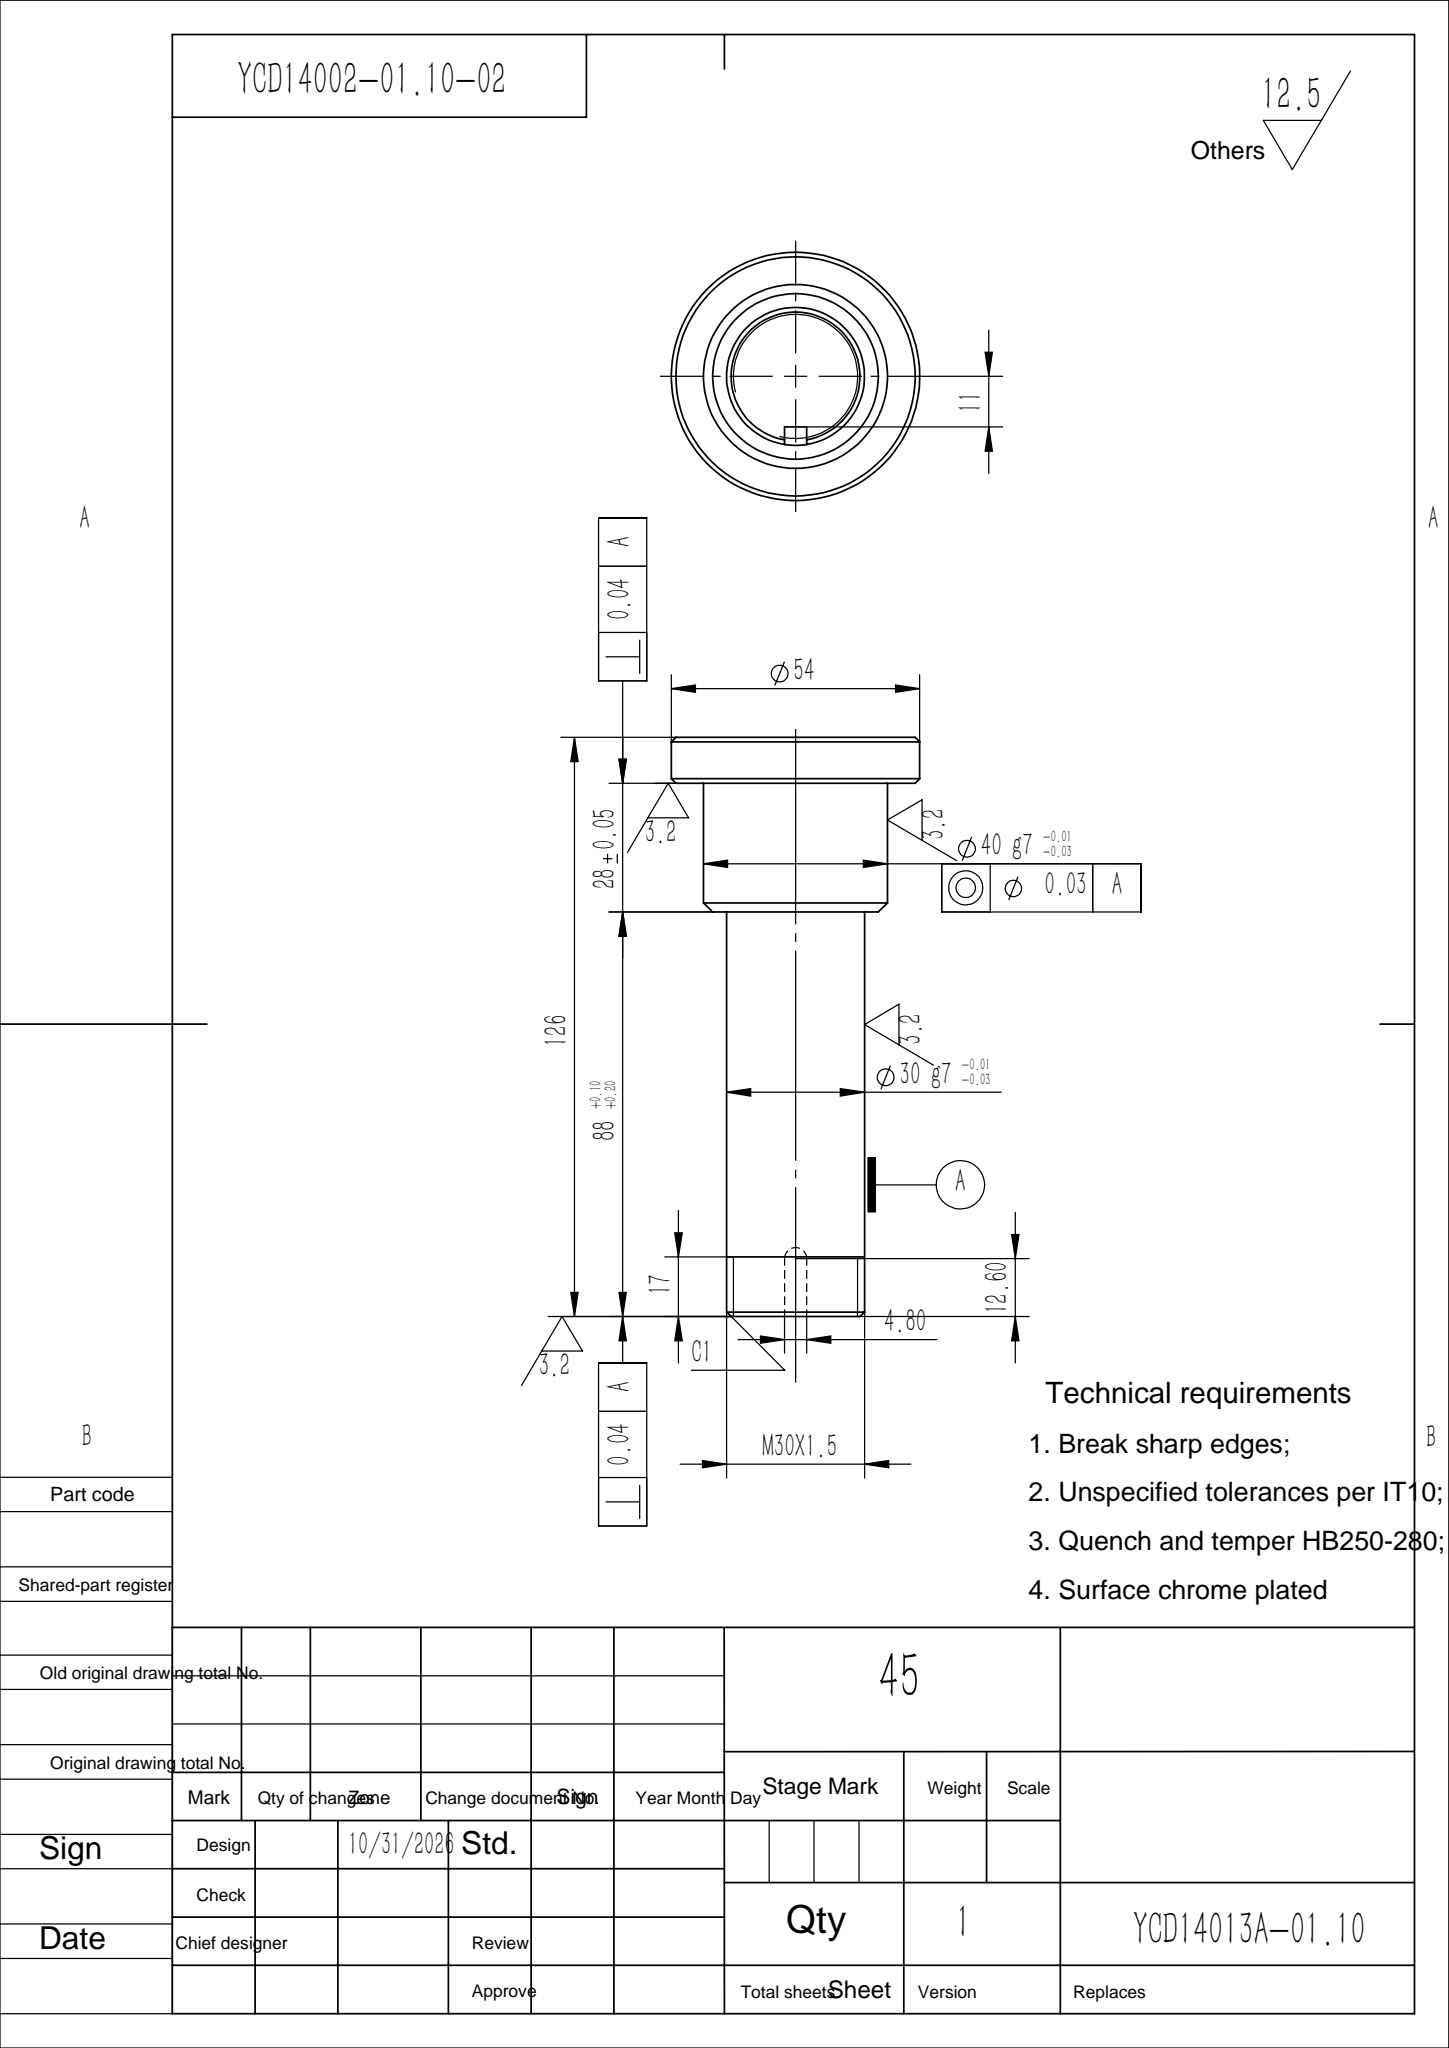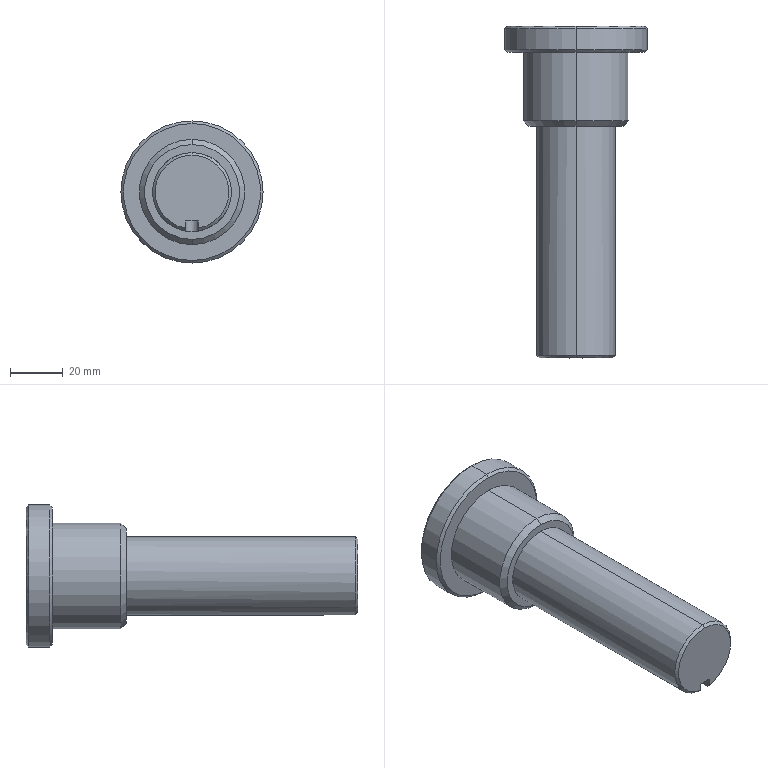Part | SolidWorks | features ICE 4, Chamfer 2, Extrusion 1 | 1 solid | 22 faces | box 54 x 126 x 54 mm | volume 119564 mm3 | cone 8 | cylinder 7 | plane 7 | commonest cylinder face diameters 30 x2 40 x2 54 x2 4.8 x1
STEP:
#1=CARTESIAN_POINT('',(0.,0.,-18.));
#2=VERTEX_POINT('',#1);
#3=CARTESIAN_POINT('',(0.,0.,18.));
#4=VERTEX_POINT('',#3);
#5=CARTESIAN_POINT('',(0.,0.,0.));
#6=DIRECTION('',(0.,-1.,0.));
#7=DIRECTION('',(0.,0.,1.));
#8=AXIS2_PLACEMENT_3D('',#5,#6,#7);
#9=CIRCLE('',#8,18.);
#10=EDGE_CURVE('',#2,#4,#9,.T.);
#11=ORIENTED_EDGE('',*,*,#10,.F.);
#12=CARTESIAN_POINT('',(0.,2.,-20.));
#13=VERTEX_POINT('',#12);
#14=CARTESIAN_POINT('',(0.,2.,-20.));
#15=DIRECTION('',(0.,0.7071,-0.7071));
#16=VECTOR('',#15,1000.);
#17=LINE('',#14,#16);
#18=EDGE_CURVE('',#2,#13,#17,.T.);
#19=ORIENTED_EDGE('',*,*,#18,.T.);
#20=CARTESIAN_POINT('',(0.,2.,20.));
#21=VERTEX_POINT('',#20);
#22=CARTESIAN_POINT('',(0.,2.,0.));
#23=DIRECTION('',(0.,1.,0.));
#24=DIRECTION('',(0.,0.,1.));
#25=AXIS2_PLACEMENT_3D('',#22,#23,#24);
#26=CIRCLE('',#25,20.);
#27=EDGE_CURVE('',#21,#13,#26,.T.);
#28=ORIENTED_EDGE('',*,*,#27,.F.);
#29=CARTESIAN_POINT('',(0.,2.,20.));
#30=DIRECTION('',(0.,0.7071,0.7071));
#31=VECTOR('',#30,1000.);
#32=LINE('',#29,#31);
#33=EDGE_CURVE('',#4,#21,#32,.T.);
#34=ORIENTED_EDGE('',*,*,#33,.F.);
#35=EDGE_LOOP('',(#11,#19,#28,#34));
#36=FACE_OUTER_BOUND('',#35,.T.);
#37=CARTESIAN_POINT('',(0.,2.,0.));
#38=DIRECTION('',(0.,1.,0.));
#39=DIRECTION('',(0.,0.,1.));
#40=AXIS2_PLACEMENT_3D('',#37,#38,#39);
#41=CONICAL_SURFACE('',#40,20.,0.7854);
#42=ADVANCED_FACE('',(#36),#41,.T.);
#43=CARTESIAN_POINT('',(0.,38.,26.));
#44=VERTEX_POINT('',#43);
#45=CARTESIAN_POINT('',(0.,38.,-26.));
#46=VERTEX_POINT('',#45);
#47=CARTESIAN_POINT('',(0.,38.,0.));
#48=DIRECTION('',(0.,1.,0.));
#49=DIRECTION('',(0.,0.,1.));
#50=AXIS2_PLACEMENT_3D('',#47,#48,#49);
#51=CIRCLE('',#50,26.);
#52=EDGE_CURVE('',#44,#46,#51,.T.);
#53=ORIENTED_EDGE('',*,*,#52,.F.);
#54=CARTESIAN_POINT('',(0.,37.,27.));
#55=VERTEX_POINT('',#54);
#56=CARTESIAN_POINT('',(0.,38.,26.));
#57=DIRECTION('',(0.,-0.7071,0.7071));
#58=VECTOR('',#57,1000.);
#59=LINE('',#56,#58);
#60=EDGE_CURVE('',#44,#55,#59,.T.);
#61=ORIENTED_EDGE('',*,*,#60,.T.);
#62=CARTESIAN_POINT('',(0.,37.,-27.));
#63=VERTEX_POINT('',#62);
#64=CARTESIAN_POINT('',(0.,37.,0.));
#65=DIRECTION('',(0.,-1.,0.));
#66=DIRECTION('',(0.,0.,1.));
#67=AXIS2_PLACEMENT_3D('',#64,#65,#66);
#68=CIRCLE('',#67,27.);
#69=EDGE_CURVE('',#63,#55,#68,.T.);
#70=ORIENTED_EDGE('',*,*,#69,.F.);
#71=CARTESIAN_POINT('',(0.,38.,-26.));
#72=DIRECTION('',(0.,-0.7071,-0.7071));
#73=VECTOR('',#72,1000.);
#74=LINE('',#71,#73);
#75=EDGE_CURVE('',#46,#63,#74,.T.);
#76=ORIENTED_EDGE('',*,*,#75,.F.);
#77=EDGE_LOOP('',(#53,#61,#70,#76));
#78=FACE_OUTER_BOUND('',#77,.T.);
#79=CARTESIAN_POINT('',(0.,38.,0.));
#80=DIRECTION('',(0.,-1.,0.));
#81=DIRECTION('',(0.,0.,-1.));
#82=AXIS2_PLACEMENT_3D('',#79,#80,#81);
#83=CONICAL_SURFACE('',#82,26.,0.7854);
#84=ADVANCED_FACE('',(#78),#83,.T.);
#85=CARTESIAN_POINT('',(0.,28.,-26.));
#86=VERTEX_POINT('',#85);
#87=CARTESIAN_POINT('',(0.,28.,26.));
#88=VERTEX_POINT('',#87);
#89=CARTESIAN_POINT('',(0.,28.,0.));
#90=DIRECTION('',(0.,-1.,0.));
#91=DIRECTION('',(0.,0.,1.));
#92=AXIS2_PLACEMENT_3D('',#89,#90,#91);
#93=CIRCLE('',#92,26.);
#94=EDGE_CURVE('',#86,#88,#93,.T.);
#95=ORIENTED_EDGE('',*,*,#94,.F.);
#96=CARTESIAN_POINT('',(0.,29.,-27.));
#97=VERTEX_POINT('',#96);
#98=CARTESIAN_POINT('',(0.,29.,-27.));
#99=DIRECTION('',(0.,0.7071,-0.7071));
#100=VECTOR('',#99,1000.);
#101=LINE('',#98,#100);
#102=EDGE_CURVE('',#86,#97,#101,.T.);
#103=ORIENTED_EDGE('',*,*,#102,.T.);
#104=CARTESIAN_POINT('',(0.,29.,27.));
#105=VERTEX_POINT('',#104);
#106=CARTESIAN_POINT('',(0.,29.,0.));
#107=DIRECTION('',(0.,1.,0.));
#108=DIRECTION('',(0.,0.,1.));
#109=AXIS2_PLACEMENT_3D('',#106,#107,#108);
#110=CIRCLE('',#109,27.);
#111=EDGE_CURVE('',#105,#97,#110,.T.);
#112=ORIENTED_EDGE('',*,*,#111,.F.);
#113=CARTESIAN_POINT('',(0.,29.,27.));
#114=DIRECTION('',(0.,0.7071,0.7071));
#115=VECTOR('',#114,1000.);
#116=LINE('',#113,#115);
#117=EDGE_CURVE('',#88,#105,#116,.T.);
#118=ORIENTED_EDGE('',*,*,#117,.F.);
#119=EDGE_LOOP('',(#95,#103,#112,#118));
#120=FACE_OUTER_BOUND('',#119,.T.);
#121=CARTESIAN_POINT('',(0.,29.,0.));
#122=DIRECTION('',(0.,1.,0.));
#123=DIRECTION('',(0.,0.,1.));
#124=AXIS2_PLACEMENT_3D('',#121,#122,#123);
#125=CONICAL_SURFACE('',#124,27.,0.7854);
#126=ADVANCED_FACE('',(#120),#125,.T.);
#127=CARTESIAN_POINT('',(0.,-88.,14.));
#128=VERTEX_POINT('',#127);
#129=CARTESIAN_POINT('',(-2.4,-88.,-13.793));
#130=VERTEX_POINT('',#129);
#131=CARTESIAN_POINT('',(0.,-88.,0.));
#132=DIRECTION('',(0.,-1.,0.));
#133=DIRECTION('',(0.,0.,-1.));
#134=AXIS2_PLACEMENT_3D('',#131,#132,#133);
#135=CIRCLE('',#134,14.);
#136=EDGE_CURVE('',#128,#130,#135,.T.);
#137=ORIENTED_EDGE('',*,*,#136,.F.);
#138=CARTESIAN_POINT('',(0.,-87.,15.));
#139=VERTEX_POINT('',#138);
#140=CARTESIAN_POINT('',(0.,-88.,14.));
#141=DIRECTION('',(0.,0.7071,0.7071));
#142=VECTOR('',#141,1000.);
#143=LINE('',#140,#142);
#144=EDGE_CURVE('',#128,#139,#143,.T.);
#145=ORIENTED_EDGE('',*,*,#144,.T.);
#146=CARTESIAN_POINT('',(-2.4,-87.,-14.807));
#147=VERTEX_POINT('',#146);
#148=CARTESIAN_POINT('',(0.,-87.,0.));
#149=DIRECTION('',(0.,1.,0.));
#150=DIRECTION('',(0.,0.,-1.));
#151=AXIS2_PLACEMENT_3D('',#148,#149,#150);
#152=CIRCLE('',#151,15.);
#153=EDGE_CURVE('',#147,#139,#152,.T.);
#154=ORIENTED_EDGE('',*,*,#153,.F.);
#155=CARTESIAN_POINT('',(-2.4,-88.,-13.793));
#156=CARTESIAN_POINT('',(-2.4,-87.667,-14.131));
#157=CARTESIAN_POINT('',(-2.4,-87.333,-14.469));
#158=CARTESIAN_POINT('',(-2.4,-87.,-14.807));
#159=B_SPLINE_CURVE_WITH_KNOTS('',3,(#155,#156,#157,#158),.UNSPECIFIED.,.F.,.F.,(4,4),(0.006945,0.00837),.UNSPECIFIED.);
#160=EDGE_CURVE('',#130,#147,#159,.T.);
#161=ORIENTED_EDGE('',*,*,#160,.F.);
#162=EDGE_LOOP('',(#137,#145,#154,#161));
#163=FACE_OUTER_BOUND('',#162,.T.);
#164=CARTESIAN_POINT('',(0.,-88.,0.));
#165=DIRECTION('',(0.,1.,0.));
#166=DIRECTION('',(0.,0.,1.));
#167=AXIS2_PLACEMENT_3D('',#164,#165,#166);
#168=CONICAL_SURFACE('',#167,14.,0.7854);
#169=ADVANCED_FACE('',(#163),#168,.T.);
#170=CARTESIAN_POINT('',(2.4,-75.4,-14.807));
#171=VERTEX_POINT('',#170);
#172=CARTESIAN_POINT('',(0.,-73.,-15.));
#173=VERTEX_POINT('',#172);
#174=CARTESIAN_POINT('',(2.4,-75.4,-14.807));
#175=CARTESIAN_POINT('',(2.4,-75.241,-14.807));
#176=CARTESIAN_POINT('',(2.384,-75.085,-14.809));
#177=CARTESIAN_POINT('',(2.323,-74.778,-14.819));
#178=CARTESIAN_POINT('',(2.277,-74.625,-14.826));
#179=CARTESIAN_POINT('',(2.156,-74.335,-14.844));
#180=CARTESIAN_POINT('',(2.083,-74.197,-14.855));
#181=CARTESIAN_POINT('',(1.908,-73.936,-14.878));
#182=CARTESIAN_POINT('',(1.807,-73.813,-14.891));
#183=CARTESIAN_POINT('',(1.475,-73.481,-14.929));
#184=CARTESIAN_POINT('',(1.208,-73.303,-14.954));
#185=CARTESIAN_POINT('',(0.7745,-73.123,-14.981));
#186=CARTESIAN_POINT('',(0.6228,-73.077,-14.988));
#187=CARTESIAN_POINT('',(0.3128,-73.015,-14.998));
#188=CARTESIAN_POINT('',(0.1569,-73.,-15.));
#189=CARTESIAN_POINT('',(0.,-73.,-15.));
#190=B_SPLINE_CURVE_WITH_KNOTS('',3,(#174,#175,#176,#177,#178,#179,#180,#181,#182,#183,#184,#185,#186,#187,#188,#189),.UNSPECIFIED.,.F.,.F.,(4,2,2,2,2,2,2,4),(0.,0.0004698,0.0009397,0.00141,0.001879,0.002819,0.003289,0.003759),.UNSPECIFIED.);
#191=EDGE_CURVE('',#171,#173,#190,.T.);
#192=ORIENTED_EDGE('',*,*,#191,.T.);
#193=CARTESIAN_POINT('',(0.,0.,-15.));
#194=VERTEX_POINT('',#193);
#195=CARTESIAN_POINT('',(0.,-88.,-15.));
#196=DIRECTION('',(0.,1.,0.));
#197=VECTOR('',#196,1000.);
#198=LINE('',#195,#197);
#199=EDGE_CURVE('',#173,#194,#198,.T.);
#200=ORIENTED_EDGE('',*,*,#199,.T.);
#201=CARTESIAN_POINT('',(0.,0.,15.));
#202=VERTEX_POINT('',#201);
#203=CARTESIAN_POINT('',(0.,0.,0.));
#204=DIRECTION('',(0.,-1.,0.));
#205=DIRECTION('',(0.,0.,1.));
#206=AXIS2_PLACEMENT_3D('',#203,#204,#205);
#207=CIRCLE('',#206,15.);
#208=EDGE_CURVE('',#194,#202,#207,.T.);
#209=ORIENTED_EDGE('',*,*,#208,.T.);
#210=CARTESIAN_POINT('',(0.,-88.,15.));
#211=DIRECTION('',(0.,1.,0.));
#212=VECTOR('',#211,1000.);
#213=LINE('',#210,#212);
#214=EDGE_CURVE('',#139,#202,#213,.T.);
#215=ORIENTED_EDGE('',*,*,#214,.F.);
#216=CARTESIAN_POINT('',(2.4,-87.,-14.807));
#217=VERTEX_POINT('',#216);
#218=CARTESIAN_POINT('',(0.,-87.,0.));
#219=DIRECTION('',(0.,1.,0.));
#220=DIRECTION('',(0.,0.,-1.));
#221=AXIS2_PLACEMENT_3D('',#218,#219,#220);
#222=CIRCLE('',#221,15.);
#223=EDGE_CURVE('',#139,#217,#222,.T.);
#224=ORIENTED_EDGE('',*,*,#223,.T.);
#225=CARTESIAN_POINT('',(2.4,-88.,-14.807));
#226=DIRECTION('',(0.,1.,0.));
#227=VECTOR('',#226,1000.);
#228=LINE('',#225,#227);
#229=EDGE_CURVE('',#217,#171,#228,.T.);
#230=ORIENTED_EDGE('',*,*,#229,.T.);
#231=EDGE_LOOP('',(#192,#200,#209,#215,#224,#230));
#232=FACE_OUTER_BOUND('',#231,.T.);
#233=CARTESIAN_POINT('',(0.,-88.,0.));
#234=DIRECTION('',(0.,1.,0.));
#235=DIRECTION('',(0.,0.,1.));
#236=AXIS2_PLACEMENT_3D('',#233,#234,#235);
#237=CYLINDRICAL_SURFACE('',#236,15.);
#238=ADVANCED_FACE('',(#232),#237,.T.);
#239=ORIENTED_EDGE('',*,*,#69,.T.);
#240=CARTESIAN_POINT('',(0.,38.,27.));
#241=DIRECTION('',(0.,-1.,0.));
#242=VECTOR('',#241,1000.);
#243=LINE('',#240,#242);
#244=EDGE_CURVE('',#55,#105,#243,.T.);
#245=ORIENTED_EDGE('',*,*,#244,.T.);
#246=ORIENTED_EDGE('',*,*,#111,.T.);
#247=CARTESIAN_POINT('',(0.,38.,-27.));
#248=DIRECTION('',(0.,-1.,0.));
#249=VECTOR('',#248,1000.);
#250=LINE('',#247,#249);
#251=EDGE_CURVE('',#63,#97,#250,.T.);
#252=ORIENTED_EDGE('',*,*,#251,.F.);
#253=EDGE_LOOP('',(#239,#245,#246,#252));
#254=FACE_OUTER_BOUND('',#253,.T.);
#255=CARTESIAN_POINT('',(0.,38.,0.));
#256=DIRECTION('',(0.,-1.,0.));
#257=DIRECTION('',(0.,0.,-1.));
#258=AXIS2_PLACEMENT_3D('',#255,#256,#257);
#259=CYLINDRICAL_SURFACE('',#258,27.);
#260=ADVANCED_FACE('',(#254),#259,.T.);
#261=CARTESIAN_POINT('',(0.,28.,20.));
#262=VERTEX_POINT('',#261);
#263=CARTESIAN_POINT('',(0.,28.,-20.));
#264=VERTEX_POINT('',#263);
#265=CARTESIAN_POINT('',(0.,28.,0.));
#266=DIRECTION('',(0.,1.,0.));
#267=DIRECTION('',(0.,0.,1.));
#268=AXIS2_PLACEMENT_3D('',#265,#266,#267);
#269=CIRCLE('',#268,20.);
#270=EDGE_CURVE('',#262,#264,#269,.T.);
#271=ORIENTED_EDGE('',*,*,#270,.F.);
#272=CARTESIAN_POINT('',(0.,28.,20.));
#273=DIRECTION('',(0.,-1.,0.));
#274=VECTOR('',#273,1000.);
#275=LINE('',#272,#274);
#276=EDGE_CURVE('',#262,#21,#275,.T.);
#277=ORIENTED_EDGE('',*,*,#276,.T.);
#278=ORIENTED_EDGE('',*,*,#27,.T.);
#279=CARTESIAN_POINT('',(0.,28.,-20.));
#280=DIRECTION('',(0.,-1.,0.));
#281=VECTOR('',#280,1000.);
#282=LINE('',#279,#281);
#283=EDGE_CURVE('',#264,#13,#282,.T.);
#284=ORIENTED_EDGE('',*,*,#283,.F.);
#285=EDGE_LOOP('',(#271,#277,#278,#284));
#286=FACE_OUTER_BOUND('',#285,.T.);
#287=CARTESIAN_POINT('',(0.,28.,0.));
#288=DIRECTION('',(0.,-1.,0.));
#289=DIRECTION('',(0.,0.,-1.));
#290=AXIS2_PLACEMENT_3D('',#287,#288,#289);
#291=CYLINDRICAL_SURFACE('',#290,20.);
#292=ADVANCED_FACE('',(#286),#291,.T.);
#293=CARTESIAN_POINT('',(0.,0.,0.));
#294=DIRECTION('',(0.,-1.,0.));
#295=DIRECTION('',(0.,0.,1.));
#296=AXIS2_PLACEMENT_3D('',#293,#294,#295);
#297=CIRCLE('',#296,18.);
#298=EDGE_CURVE('',#4,#2,#297,.T.);
#299=ORIENTED_EDGE('',*,*,#298,.T.);
#300=ORIENTED_EDGE('',*,*,#10,.T.);
#301=EDGE_LOOP('',(#299,#300));
#302=FACE_OUTER_BOUND('',#301,.T.);
#303=CARTESIAN_POINT('',(0.,0.,0.));
#304=DIRECTION('',(0.,-1.,0.));
#305=DIRECTION('',(0.,0.,1.));
#306=AXIS2_PLACEMENT_3D('',#303,#304,#305);
#307=CIRCLE('',#306,15.);
#308=EDGE_CURVE('',#202,#194,#307,.T.);
#309=ORIENTED_EDGE('',*,*,#308,.F.);
#310=ORIENTED_EDGE('',*,*,#208,.F.);
#311=EDGE_LOOP('',(#309,#310));
#312=FACE_BOUND('',#311,.T.);
#313=CARTESIAN_POINT('',(0.,0.,0.));
#314=DIRECTION('',(0.,1.,0.));
#315=DIRECTION('',(0.,0.,1.));
#316=AXIS2_PLACEMENT_3D('',#313,#314,#315);
#317=PLANE('',#316);
#318=ADVANCED_FACE('',(#302,#312),#317,.F.);
#319=ORIENTED_EDGE('',*,*,#276,.F.);
#320=CARTESIAN_POINT('',(0.,28.,0.));
#321=DIRECTION('',(0.,1.,0.));
#322=DIRECTION('',(0.,0.,1.));
#323=AXIS2_PLACEMENT_3D('',#320,#321,#322);
#324=CIRCLE('',#323,20.);
#325=EDGE_CURVE('',#264,#262,#324,.T.);
#326=ORIENTED_EDGE('',*,*,#325,.F.);
#327=ORIENTED_EDGE('',*,*,#283,.T.);
#328=CARTESIAN_POINT('',(0.,2.,0.));
#329=DIRECTION('',(0.,1.,0.));
#330=DIRECTION('',(0.,0.,1.));
#331=AXIS2_PLACEMENT_3D('',#328,#329,#330);
#332=CIRCLE('',#331,20.);
#333=EDGE_CURVE('',#13,#21,#332,.T.);
#334=ORIENTED_EDGE('',*,*,#333,.T.);
#335=EDGE_LOOP('',(#319,#326,#327,#334));
#336=FACE_OUTER_BOUND('',#335,.T.);
#337=CARTESIAN_POINT('',(0.,28.,0.));
#338=DIRECTION('',(0.,-1.,0.));
#339=DIRECTION('',(0.,0.,-1.));
#340=AXIS2_PLACEMENT_3D('',#337,#338,#339);
#341=CYLINDRICAL_SURFACE('',#340,20.);
#342=ADVANCED_FACE('',(#336),#341,.T.);
#343=CARTESIAN_POINT('',(0.,28.,0.));
#344=DIRECTION('',(0.,-1.,0.));
#345=DIRECTION('',(0.,0.,1.));
#346=AXIS2_PLACEMENT_3D('',#343,#344,#345);
#347=CIRCLE('',#346,26.);
#348=EDGE_CURVE('',#88,#86,#347,.T.);
#349=ORIENTED_EDGE('',*,*,#348,.T.);
#350=ORIENTED_EDGE('',*,*,#94,.T.);
#351=EDGE_LOOP('',(#349,#350));
#352=FACE_OUTER_BOUND('',#351,.T.);
#353=ORIENTED_EDGE('',*,*,#325,.T.);
#354=ORIENTED_EDGE('',*,*,#270,.T.);
#355=EDGE_LOOP('',(#353,#354));
#356=FACE_BOUND('',#355,.T.);
#357=CARTESIAN_POINT('',(0.,28.,0.));
#358=DIRECTION('',(0.,1.,0.));
#359=DIRECTION('',(0.,0.,1.));
#360=AXIS2_PLACEMENT_3D('',#357,#358,#359);
#361=PLANE('',#360);
#362=ADVANCED_FACE('',(#352,#356),#361,.F.);
#363=ORIENTED_EDGE('',*,*,#244,.F.);
#364=CARTESIAN_POINT('',(0.,37.,0.));
#365=DIRECTION('',(0.,-1.,0.));
#366=DIRECTION('',(0.,0.,1.));
#367=AXIS2_PLACEMENT_3D('',#364,#365,#366);
#368=CIRCLE('',#367,27.);
#369=EDGE_CURVE('',#55,#63,#368,.T.);
#370=ORIENTED_EDGE('',*,*,#369,.T.);
#371=ORIENTED_EDGE('',*,*,#251,.T.);
#372=CARTESIAN_POINT('',(0.,29.,0.));
#373=DIRECTION('',(0.,1.,0.));
#374=DIRECTION('',(0.,0.,1.));
#375=AXIS2_PLACEMENT_3D('',#372,#373,#374);
#376=CIRCLE('',#375,27.);
#377=EDGE_CURVE('',#97,#105,#376,.T.);
#378=ORIENTED_EDGE('',*,*,#377,.T.);
#379=EDGE_LOOP('',(#363,#370,#371,#378));
#380=FACE_OUTER_BOUND('',#379,.T.);
#381=CARTESIAN_POINT('',(0.,38.,0.));
#382=DIRECTION('',(0.,-1.,0.));
#383=DIRECTION('',(0.,0.,-1.));
#384=AXIS2_PLACEMENT_3D('',#381,#382,#383);
#385=CYLINDRICAL_SURFACE('',#384,27.);
#386=ADVANCED_FACE('',(#380),#385,.T.);
#387=CARTESIAN_POINT('',(0.,38.,0.));
#388=DIRECTION('',(0.,1.,0.));
#389=DIRECTION('',(0.,0.,1.));
#390=AXIS2_PLACEMENT_3D('',#387,#388,#389);
#391=CIRCLE('',#390,26.);
#392=EDGE_CURVE('',#46,#44,#391,.T.);
#393=ORIENTED_EDGE('',*,*,#392,.T.);
#394=ORIENTED_EDGE('',*,*,#52,.T.);
#395=EDGE_LOOP('',(#393,#394));
#396=FACE_OUTER_BOUND('',#395,.T.);
#397=CARTESIAN_POINT('',(0.,38.,0.));
#398=DIRECTION('',(0.,1.,0.));
#399=DIRECTION('',(0.,0.,1.));
#400=AXIS2_PLACEMENT_3D('',#397,#398,#399);
#401=PLANE('',#400);
#402=ADVANCED_FACE('',(#396),#401,.T.);
#403=ORIENTED_EDGE('',*,*,#199,.F.);
#404=CARTESIAN_POINT('',(-2.4,-75.4,-14.807));
#405=VERTEX_POINT('',#404);
#406=CARTESIAN_POINT('',(0.,-73.,-15.));
#407=CARTESIAN_POINT('',(-0.1567,-73.,-15.));
#408=CARTESIAN_POINT('',(-0.3159,-73.016,-14.997));
#409=CARTESIAN_POINT('',(-0.6237,-73.077,-14.988));
#410=CARTESIAN_POINT('',(-0.7733,-73.123,-14.981));
#411=CARTESIAN_POINT('',(-1.064,-73.243,-14.963));
#412=CARTESIAN_POINT('',(-1.204,-73.318,-14.952));
#413=CARTESIAN_POINT('',(-1.464,-73.492,-14.929));
#414=CARTESIAN_POINT('',(-1.585,-73.591,-14.916));
#415=CARTESIAN_POINT('',(-1.808,-73.814,-14.891));
#416=CARTESIAN_POINT('',(-1.907,-73.935,-14.878));
#417=CARTESIAN_POINT('',(-2.081,-74.195,-14.855));
#418=CARTESIAN_POINT('',(-2.156,-74.335,-14.844));
#419=CARTESIAN_POINT('',(-2.277,-74.625,-14.826));
#420=CARTESIAN_POINT('',(-2.322,-74.775,-14.819));
#421=CARTESIAN_POINT('',(-2.384,-75.082,-14.809));
#422=CARTESIAN_POINT('',(-2.4,-75.241,-14.807));
#423=CARTESIAN_POINT('',(-2.4,-75.4,-14.807));
#424=B_SPLINE_CURVE_WITH_KNOTS('',3,(#406,#407,#408,#409,#410,#411,#412,#413,#414,#415,#416,#417,#418,#419,#420,#421,#422,#423),.UNSPECIFIED.,.F.,.F.,(4,2,2,2,2,2,2,2,4),(0.003759,0.004228,0.004697,0.005167,0.005636,0.006106,0.006575,0.007044,0.007514),.UNSPECIFIED.);
#425=EDGE_CURVE('',#173,#405,#424,.T.);
#426=ORIENTED_EDGE('',*,*,#425,.T.);
#427=CARTESIAN_POINT('',(-2.4,-88.,-14.807));
#428=DIRECTION('',(0.,-1.,0.));
#429=VECTOR('',#428,1000.);
#430=LINE('',#427,#429);
#431=EDGE_CURVE('',#405,#147,#430,.T.);
#432=ORIENTED_EDGE('',*,*,#431,.T.);
#433=ORIENTED_EDGE('',*,*,#153,.T.);
#434=ORIENTED_EDGE('',*,*,#214,.T.);
#435=ORIENTED_EDGE('',*,*,#308,.T.);
#436=EDGE_LOOP('',(#403,#426,#432,#433,#434,#435));
#437=FACE_OUTER_BOUND('',#436,.T.);
#438=CARTESIAN_POINT('',(0.,-88.,0.));
#439=DIRECTION('',(0.,1.,0.));
#440=DIRECTION('',(0.,0.,1.));
#441=AXIS2_PLACEMENT_3D('',#438,#439,#440);
#442=CYLINDRICAL_SURFACE('',#441,15.);
#443=ADVANCED_FACE('',(#437),#442,.T.);
#444=CARTESIAN_POINT('',(2.4,-88.,-13.793));
#445=VERTEX_POINT('',#444);
#446=CARTESIAN_POINT('',(2.4,-88.,-11.));
#447=VERTEX_POINT('',#446);
#448=CARTESIAN_POINT('',(2.4,-88.,0.));
#449=DIRECTION('',(0.,0.,1.));
#450=VECTOR('',#449,1000.);
#451=LINE('',#448,#450);
#452=EDGE_CURVE('',#445,#447,#451,.T.);
#453=ORIENTED_EDGE('',*,*,#452,.F.);
#454=CARTESIAN_POINT('',(0.,-88.,0.));
#455=DIRECTION('',(0.,-1.,0.));
#456=DIRECTION('',(0.,0.,-1.));
#457=AXIS2_PLACEMENT_3D('',#454,#455,#456);
#458=CIRCLE('',#457,14.);
#459=EDGE_CURVE('',#445,#128,#458,.T.);
#460=ORIENTED_EDGE('',*,*,#459,.T.);
#461=ORIENTED_EDGE('',*,*,#136,.T.);
#462=CARTESIAN_POINT('',(-2.4,-88.,-11.));
#463=VERTEX_POINT('',#462);
#464=CARTESIAN_POINT('',(-2.4,-88.,0.));
#465=DIRECTION('',(0.,0.,-1.));
#466=VECTOR('',#465,1000.);
#467=LINE('',#464,#466);
#468=EDGE_CURVE('',#463,#130,#467,.T.);
#469=ORIENTED_EDGE('',*,*,#468,.F.);
#470=CARTESIAN_POINT('',(0.,-88.,-11.));
#471=DIRECTION('',(-1.,0.,0.));
#472=VECTOR('',#471,1000.);
#473=LINE('',#470,#472);
#474=EDGE_CURVE('',#447,#463,#473,.T.);
#475=ORIENTED_EDGE('',*,*,#474,.F.);
#476=EDGE_LOOP('',(#453,#460,#461,#469,#475));
#477=FACE_OUTER_BOUND('',#476,.T.);
#478=CARTESIAN_POINT('',(0.,-88.,0.));
#479=DIRECTION('',(0.,-1.,0.));
#480=DIRECTION('',(0.,0.,-1.));
#481=AXIS2_PLACEMENT_3D('',#478,#479,#480);
#482=PLANE('',#481);
#483=ADVANCED_FACE('',(#477),#482,.T.);
#484=ORIENTED_EDGE('',*,*,#144,.F.);
#485=ORIENTED_EDGE('',*,*,#459,.F.);
#486=CARTESIAN_POINT('',(2.4,-87.,-14.807));
#487=CARTESIAN_POINT('',(2.4,-87.333,-14.469));
#488=CARTESIAN_POINT('',(2.4,-87.667,-14.131));
#489=CARTESIAN_POINT('',(2.4,-88.,-13.793));
#490=B_SPLINE_CURVE_WITH_KNOTS('',3,(#486,#487,#488,#489),.UNSPECIFIED.,.F.,.F.,(4,4),(0.007231,0.008655),.UNSPECIFIED.);
#491=EDGE_CURVE('',#217,#445,#490,.T.);
#492=ORIENTED_EDGE('',*,*,#491,.F.);
#493=ORIENTED_EDGE('',*,*,#223,.F.);
#494=EDGE_LOOP('',(#484,#485,#492,#493));
#495=FACE_OUTER_BOUND('',#494,.T.);
#496=CARTESIAN_POINT('',(0.,-88.,0.));
#497=DIRECTION('',(0.,1.,0.));
#498=DIRECTION('',(0.,0.,1.));
#499=AXIS2_PLACEMENT_3D('',#496,#497,#498);
#500=CONICAL_SURFACE('',#499,14.,0.7854);
#501=ADVANCED_FACE('',(#495),#500,.T.);
#502=ORIENTED_EDGE('',*,*,#102,.F.);
#503=ORIENTED_EDGE('',*,*,#348,.F.);
#504=ORIENTED_EDGE('',*,*,#117,.T.);
#505=ORIENTED_EDGE('',*,*,#377,.F.);
#506=EDGE_LOOP('',(#502,#503,#504,#505));
#507=FACE_OUTER_BOUND('',#506,.T.);
#508=CARTESIAN_POINT('',(0.,29.,0.));
#509=DIRECTION('',(0.,1.,0.));
#510=DIRECTION('',(0.,0.,1.));
#511=AXIS2_PLACEMENT_3D('',#508,#509,#510);
#512=CONICAL_SURFACE('',#511,27.,0.7854);
#513=ADVANCED_FACE('',(#507),#512,.T.);
#514=ORIENTED_EDGE('',*,*,#60,.F.);
#515=ORIENTED_EDGE('',*,*,#392,.F.);
#516=ORIENTED_EDGE('',*,*,#75,.T.);
#517=ORIENTED_EDGE('',*,*,#369,.F.);
#518=EDGE_LOOP('',(#514,#515,#516,#517));
#519=FACE_OUTER_BOUND('',#518,.T.);
#520=CARTESIAN_POINT('',(0.,38.,0.));
#521=DIRECTION('',(0.,-1.,0.));
#522=DIRECTION('',(0.,0.,-1.));
#523=AXIS2_PLACEMENT_3D('',#520,#521,#522);
#524=CONICAL_SURFACE('',#523,26.,0.7854);
#525=ADVANCED_FACE('',(#519),#524,.T.);
#526=ORIENTED_EDGE('',*,*,#18,.F.);
#527=ORIENTED_EDGE('',*,*,#298,.F.);
#528=ORIENTED_EDGE('',*,*,#33,.T.);
#529=ORIENTED_EDGE('',*,*,#333,.F.);
#530=EDGE_LOOP('',(#526,#527,#528,#529));
#531=FACE_OUTER_BOUND('',#530,.T.);
#532=CARTESIAN_POINT('',(0.,2.,0.));
#533=DIRECTION('',(0.,1.,0.));
#534=DIRECTION('',(0.,0.,1.));
#535=AXIS2_PLACEMENT_3D('',#532,#533,#534);
#536=CONICAL_SURFACE('',#535,20.,0.7854);
#537=ADVANCED_FACE('',(#531),#536,.T.);
#538=CARTESIAN_POINT('',(2.4,-75.4,-11.));
#539=VERTEX_POINT('',#538);
#540=CARTESIAN_POINT('',(2.4,-75.4,-22.));
#541=DIRECTION('',(0.,0.,1.));
#542=VECTOR('',#541,1000.);
#543=LINE('',#540,#542);
#544=EDGE_CURVE('',#171,#539,#543,.T.);
#545=ORIENTED_EDGE('',*,*,#544,.T.);
#546=CARTESIAN_POINT('',(-2.4,-75.4,-11.));
#547=VERTEX_POINT('',#546);
#548=CARTESIAN_POINT('',(0.,-75.4,-11.));
#549=DIRECTION('',(0.,0.,1.));
#550=DIRECTION('',(1.,0.,0.));
#551=AXIS2_PLACEMENT_3D('',#548,#549,#550);
#552=CIRCLE('',#551,2.4);
#553=EDGE_CURVE('',#539,#547,#552,.T.);
#554=ORIENTED_EDGE('',*,*,#553,.T.);
#555=CARTESIAN_POINT('',(-2.4,-75.4,-22.));
#556=DIRECTION('',(0.,0.,1.));
#557=VECTOR('',#556,1000.);
#558=LINE('',#555,#557);
#559=EDGE_CURVE('',#405,#547,#558,.T.);
#560=ORIENTED_EDGE('',*,*,#559,.F.);
#561=ORIENTED_EDGE('',*,*,#425,.F.);
#562=ORIENTED_EDGE('',*,*,#191,.F.);
#563=EDGE_LOOP('',(#545,#554,#560,#561,#562));
#564=FACE_OUTER_BOUND('',#563,.T.);
#565=CARTESIAN_POINT('',(0.,-75.4,-22.));
#566=DIRECTION('',(0.,0.,1.));
#567=DIRECTION('',(1.,0.,0.));
#568=AXIS2_PLACEMENT_3D('',#565,#566,#567);
#569=CYLINDRICAL_SURFACE('',#568,2.4);
#570=ADVANCED_FACE('',(#564),#569,.F.);
#571=ORIENTED_EDGE('',*,*,#491,.T.);
#572=ORIENTED_EDGE('',*,*,#452,.T.);
#573=CARTESIAN_POINT('',(2.4,-100.6,-11.));
#574=DIRECTION('',(0.,1.,0.));
#575=VECTOR('',#574,1000.);
#576=LINE('',#573,#575);
#577=EDGE_CURVE('',#447,#539,#576,.T.);
#578=ORIENTED_EDGE('',*,*,#577,.T.);
#579=ORIENTED_EDGE('',*,*,#544,.F.);
#580=ORIENTED_EDGE('',*,*,#229,.F.);
#581=EDGE_LOOP('',(#571,#572,#578,#579,#580));
#582=FACE_OUTER_BOUND('',#581,.T.);
#583=CARTESIAN_POINT('',(2.4,-100.6,-22.));
#584=DIRECTION('',(1.,0.,0.));
#585=DIRECTION('',(0.,1.,0.));
#586=AXIS2_PLACEMENT_3D('',#583,#584,#585);
#587=PLANE('',#586);
#588=ADVANCED_FACE('',(#582),#587,.F.);
#589=ORIENTED_EDGE('',*,*,#559,.T.);
#590=CARTESIAN_POINT('',(-2.4,-100.6,-11.));
#591=DIRECTION('',(0.,-1.,0.));
#592=VECTOR('',#591,1000.);
#593=LINE('',#590,#592);
#594=EDGE_CURVE('',#547,#463,#593,.T.);
#595=ORIENTED_EDGE('',*,*,#594,.T.);
#596=ORIENTED_EDGE('',*,*,#468,.T.);
#597=ORIENTED_EDGE('',*,*,#160,.T.);
#598=ORIENTED_EDGE('',*,*,#431,.F.);
#599=EDGE_LOOP('',(#589,#595,#596,#597,#598));
#600=FACE_OUTER_BOUND('',#599,.T.);
#601=CARTESIAN_POINT('',(-2.4,-100.6,-22.));
#602=DIRECTION('',(-1.,0.,0.));
#603=DIRECTION('',(0.,-1.,0.));
#604=AXIS2_PLACEMENT_3D('',#601,#602,#603);
#605=PLANE('',#604);
#606=ADVANCED_FACE('',(#600),#605,.F.);
#607=ORIENTED_EDGE('',*,*,#474,.T.);
#608=ORIENTED_EDGE('',*,*,#594,.F.);
#609=ORIENTED_EDGE('',*,*,#553,.F.);
#610=ORIENTED_EDGE('',*,*,#577,.F.);
#611=EDGE_LOOP('',(#607,#608,#609,#610));
#612=FACE_OUTER_BOUND('',#611,.T.);
#613=CARTESIAN_POINT('',(0.,-75.4,-11.));
#614=DIRECTION('',(0.,0.,1.));
#615=DIRECTION('',(1.,0.,0.));
#616=AXIS2_PLACEMENT_3D('',#613,#614,#615);
#617=PLANE('',#616);
#618=ADVANCED_FACE('',(#612),#617,.F.);
#619=CLOSED_SHELL('',(#42,#84,#126,#169,#238,#260,#292,#318,#342,#362,#386,#402,#443,#483,#501,#513,#525,#537,#570,#588,#606,#618));
#620=MANIFOLD_SOLID_BREP('',#619);
#621=CARTESIAN_POINT('',(0.,0.,0.));
#622=DIRECTION('',(0.,0.,1.));
#623=DIRECTION('',(1.,0.,0.));
#624=AXIS2_PLACEMENT_3D('',#621,#622,#623);
#625=(LENGTH_UNIT()NAMED_UNIT(*)SI_UNIT(.MILLI.,.METRE.));
#626=UNCERTAINTY_MEASURE_WITH_UNIT(LENGTH_MEASURE(0.00001),#625,'','');
#627=(NAMED_UNIT(*)PLANE_ANGLE_UNIT()SI_UNIT($,.RADIAN.));
#628=(NAMED_UNIT(*)SI_UNIT($,.STERADIAN.)SOLID_ANGLE_UNIT());
#629=(GEOMETRIC_REPRESENTATION_CONTEXT(3)GLOBAL_UNCERTAINTY_ASSIGNED_CONTEXT((#626))GLOBAL_UNIT_ASSIGNED_CONTEXT((#625,#627,#628))REPRESENTATION_CONTEXT('',''));
#630=ADVANCED_BREP_SHAPE_REPRESENTATION('',(#620,#624),#629);